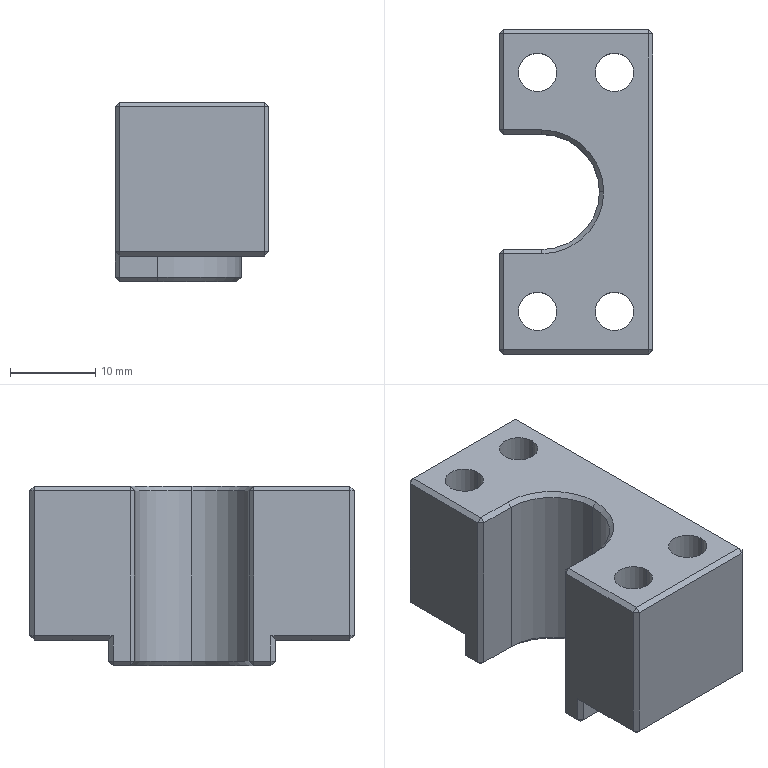Part | SolidWorks | features Chamfer 1, Cut 1, Extrusion 1, HoleWzd 1, ICE 1 | 1 solid | 81 faces | box 18 x 38 x 21 mm | volume 8331 mm3 | plane 56 | cylinder 20 | cone 5 | commonest cylinder face diameters 4.5 x8 8 x8 13.5 x2 19.5 x2